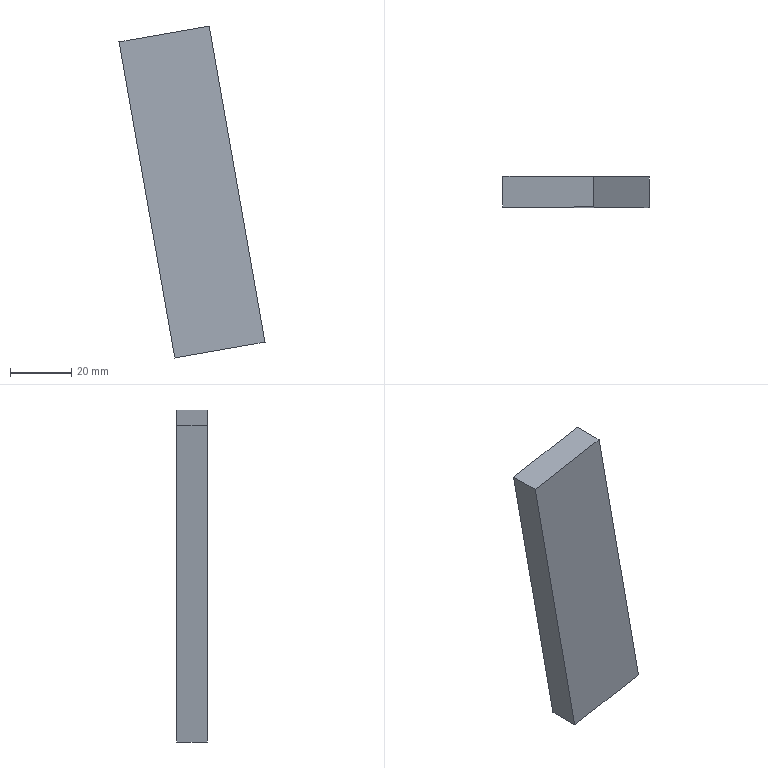Part | NX | features solid 2 | 1 solid | 6 faces | box 47.777 x 10 x 108.612 mm | volume 31499 mm3 | plane 6
STEP:
#1=CARTESIAN_POINT('',(-432.143,-70.,-8.623));
#2=VERTEX_POINT('',#1);
#3=CARTESIAN_POINT('',(-432.143,-80.,-8.623));
#4=VERTEX_POINT('',#3);
#5=CARTESIAN_POINT('',(-432.143,-70.,-8.623));
#6=DIRECTION('',(0.,1.,0.));
#7=VECTOR('',#6,1000.);
#8=LINE('',#5,#7);
#9=EDGE_CURVE('',#2,#4,#8,.F.);
#10=ORIENTED_EDGE('',*,*,#9,.F.);
#11=CARTESIAN_POINT('',(-450.376,-70.,94.779));
#12=VERTEX_POINT('',#11);
#13=CARTESIAN_POINT('',(-450.376,-70.,94.779));
#14=DIRECTION('',(0.1736,0.,-0.9848));
#15=VECTOR('',#14,1000.);
#16=LINE('',#13,#15);
#17=EDGE_CURVE('',#12,#2,#16,.T.);
#18=ORIENTED_EDGE('',*,*,#17,.F.);
#19=CARTESIAN_POINT('',(-450.376,-80.,94.779));
#20=VERTEX_POINT('',#19);
#21=CARTESIAN_POINT('',(-450.376,-70.,94.779));
#22=DIRECTION('',(0.,1.,0.));
#23=VECTOR('',#22,1000.);
#24=LINE('',#21,#23);
#25=EDGE_CURVE('',#12,#20,#24,.F.);
#26=ORIENTED_EDGE('',*,*,#25,.T.);
#27=CARTESIAN_POINT('',(-450.376,-80.,94.779));
#28=DIRECTION('',(0.1736,0.,-0.9848));
#29=VECTOR('',#28,1000.);
#30=LINE('',#27,#29);
#31=EDGE_CURVE('',#20,#4,#30,.T.);
#32=ORIENTED_EDGE('',*,*,#31,.T.);
#33=EDGE_LOOP('',(#10,#18,#26,#32));
#34=FACE_BOUND('',#33,.T.);
#35=CARTESIAN_POINT('',(-450.376,-70.,94.779));
#36=DIRECTION('',(0.9848,0.,0.1736));
#37=DIRECTION('',(0.1736,0.,-0.9848));
#38=AXIS2_PLACEMENT_3D('',#35,#36,#37);
#39=PLANE('',#38);
#40=ADVANCED_FACE('',(#34),#39,.T.);
#41=ORIENTED_EDGE('',*,*,#25,.F.);
#42=CARTESIAN_POINT('',(-479.92,-70.,89.57));
#43=VERTEX_POINT('',#42);
#44=CARTESIAN_POINT('',(-450.376,-70.,94.779));
#45=DIRECTION('',(-0.9848,0.,-0.1736));
#46=VECTOR('',#45,1000.);
#47=LINE('',#44,#46);
#48=EDGE_CURVE('',#12,#43,#47,.T.);
#49=ORIENTED_EDGE('',*,*,#48,.T.);
#50=CARTESIAN_POINT('',(-479.92,-80.,89.57));
#51=VERTEX_POINT('',#50);
#52=CARTESIAN_POINT('',(-479.92,-70.,89.57));
#53=DIRECTION('',(0.,1.,0.));
#54=VECTOR('',#53,1000.);
#55=LINE('',#52,#54);
#56=EDGE_CURVE('',#43,#51,#55,.F.);
#57=ORIENTED_EDGE('',*,*,#56,.T.);
#58=CARTESIAN_POINT('',(-450.376,-80.,94.779));
#59=DIRECTION('',(-0.9848,0.,-0.1736));
#60=VECTOR('',#59,1000.);
#61=LINE('',#58,#60);
#62=EDGE_CURVE('',#20,#51,#61,.T.);
#63=ORIENTED_EDGE('',*,*,#62,.F.);
#64=EDGE_LOOP('',(#41,#49,#57,#63));
#65=FACE_BOUND('',#64,.T.);
#66=CARTESIAN_POINT('',(-450.376,-70.,94.779));
#67=DIRECTION('',(0.1736,0.,-0.9848));
#68=DIRECTION('',(-0.9848,0.,-0.1736));
#69=AXIS2_PLACEMENT_3D('',#66,#67,#68);
#70=PLANE('',#69);
#71=ADVANCED_FACE('',(#65),#70,.F.);
#72=ORIENTED_EDGE('',*,*,#56,.F.);
#73=CARTESIAN_POINT('',(-461.687,-70.,-13.832));
#74=VERTEX_POINT('',#73);
#75=CARTESIAN_POINT('',(-479.92,-70.,89.57));
#76=DIRECTION('',(0.1736,0.,-0.9848));
#77=VECTOR('',#76,1000.);
#78=LINE('',#75,#77);
#79=EDGE_CURVE('',#43,#74,#78,.T.);
#80=ORIENTED_EDGE('',*,*,#79,.T.);
#81=CARTESIAN_POINT('',(-461.687,-80.,-13.832));
#82=VERTEX_POINT('',#81);
#83=CARTESIAN_POINT('',(-461.687,-70.,-13.832));
#84=DIRECTION('',(0.,1.,0.));
#85=VECTOR('',#84,1000.);
#86=LINE('',#83,#85);
#87=EDGE_CURVE('',#74,#82,#86,.F.);
#88=ORIENTED_EDGE('',*,*,#87,.T.);
#89=CARTESIAN_POINT('',(-479.92,-80.,89.57));
#90=DIRECTION('',(0.1736,0.,-0.9848));
#91=VECTOR('',#90,1000.);
#92=LINE('',#89,#91);
#93=EDGE_CURVE('',#51,#82,#92,.T.);
#94=ORIENTED_EDGE('',*,*,#93,.F.);
#95=EDGE_LOOP('',(#72,#80,#88,#94));
#96=FACE_BOUND('',#95,.T.);
#97=CARTESIAN_POINT('',(-479.92,-70.,89.57));
#98=DIRECTION('',(0.9848,0.,0.1736));
#99=DIRECTION('',(0.1736,0.,-0.9848));
#100=AXIS2_PLACEMENT_3D('',#97,#98,#99);
#101=PLANE('',#100);
#102=ADVANCED_FACE('',(#96),#101,.F.);
#103=CARTESIAN_POINT('',(-432.143,-70.,-8.623));
#104=DIRECTION('',(-0.9848,0.,-0.1736));
#105=VECTOR('',#104,1000.);
#106=LINE('',#103,#105);
#107=EDGE_CURVE('',#2,#74,#106,.T.);
#108=ORIENTED_EDGE('',*,*,#107,.F.);
#109=ORIENTED_EDGE('',*,*,#9,.T.);
#110=CARTESIAN_POINT('',(-432.143,-80.,-8.623));
#111=DIRECTION('',(-0.9848,0.,-0.1736));
#112=VECTOR('',#111,1000.);
#113=LINE('',#110,#112);
#114=EDGE_CURVE('',#4,#82,#113,.T.);
#115=ORIENTED_EDGE('',*,*,#114,.T.);
#116=ORIENTED_EDGE('',*,*,#87,.F.);
#117=EDGE_LOOP('',(#108,#109,#115,#116));
#118=FACE_BOUND('',#117,.T.);
#119=CARTESIAN_POINT('',(-432.143,-70.,-8.623));
#120=DIRECTION('',(0.1736,0.,-0.9848));
#121=DIRECTION('',(-0.9848,0.,-0.1736));
#122=AXIS2_PLACEMENT_3D('',#119,#120,#121);
#123=PLANE('',#122);
#124=ADVANCED_FACE('',(#118),#123,.T.);
#125=ORIENTED_EDGE('',*,*,#93,.T.);
#126=ORIENTED_EDGE('',*,*,#114,.F.);
#127=ORIENTED_EDGE('',*,*,#31,.F.);
#128=ORIENTED_EDGE('',*,*,#62,.T.);
#129=EDGE_LOOP('',(#125,#126,#127,#128));
#130=FACE_BOUND('',#129,.T.);
#131=CARTESIAN_POINT('',(-450.376,-80.,94.779));
#132=DIRECTION('',(0.,-1.,0.));
#133=DIRECTION('',(0.,0.,-1.));
#134=AXIS2_PLACEMENT_3D('',#131,#132,#133);
#135=PLANE('',#134);
#136=ADVANCED_FACE('',(#130),#135,.T.);
#137=ORIENTED_EDGE('',*,*,#79,.F.);
#138=ORIENTED_EDGE('',*,*,#48,.F.);
#139=ORIENTED_EDGE('',*,*,#17,.T.);
#140=ORIENTED_EDGE('',*,*,#107,.T.);
#141=EDGE_LOOP('',(#137,#138,#139,#140));
#142=FACE_BOUND('',#141,.T.);
#143=CARTESIAN_POINT('',(-450.376,-70.,94.779));
#144=DIRECTION('',(0.,-1.,0.));
#145=DIRECTION('',(0.,0.,-1.));
#146=AXIS2_PLACEMENT_3D('',#143,#144,#145);
#147=PLANE('',#146);
#148=ADVANCED_FACE('',(#142),#147,.F.);
#149=CLOSED_SHELL('',(#40,#71,#102,#124,#136,#148));
#150=MANIFOLD_SOLID_BREP('',#149);
#151=(LENGTH_UNIT()NAMED_UNIT(*)SI_UNIT(.MILLI.,.METRE.));
#152=UNCERTAINTY_MEASURE_WITH_UNIT(LENGTH_MEASURE(0.00001),#151,'','');
#153=(NAMED_UNIT(*)PLANE_ANGLE_UNIT()SI_UNIT($,.RADIAN.));
#154=(NAMED_UNIT(*)SI_UNIT($,.STERADIAN.)SOLID_ANGLE_UNIT());
#155=(GEOMETRIC_REPRESENTATION_CONTEXT(3)GLOBAL_UNCERTAINTY_ASSIGNED_CONTEXT((#152))GLOBAL_UNIT_ASSIGNED_CONTEXT((#151,#153,#154))REPRESENTATION_CONTEXT('',''));
#156=ADVANCED_BREP_SHAPE_REPRESENTATION('',(#150),#155);